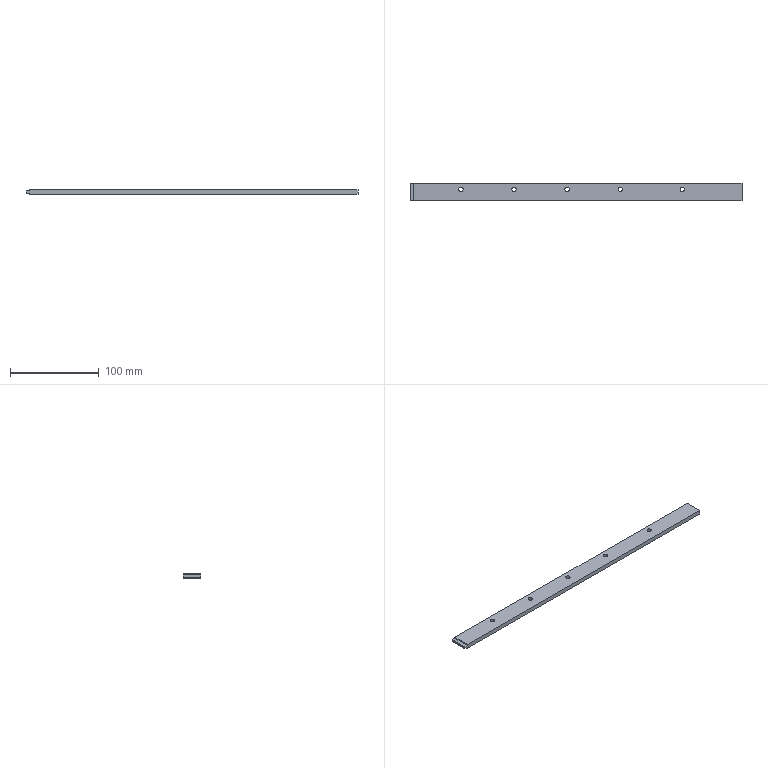Part | STEP file | slingshot press plate | 1 solid | 20 faces | box 375 x 20 x 5 mm | volume 36809 mm3 | cylinder 10 | plane 10 | commonest cylinder face diameters 5 x10
STEP:
#1=CARTESIAN_POINT('',(0.,0.,0.));
#2=DIRECTION('',(0.,0.,1.));
#3=DIRECTION('',(1.,0.,0.));
#4=AXIS2_PLACEMENT_3D('',#1,#2,#3);
#5=CARTESIAN_POINT('',(60.,-7.,0.));
#6=VERTEX_POINT('',#5);
#7=CARTESIAN_POINT('',(60.,-7.,5.));
#8=VERTEX_POINT('',#7);
#9=CARTESIAN_POINT('',(60.,-7.,5.));
#10=DIRECTION('',(0.,0.,1.));
#11=VECTOR('',#10,1.);
#12=LINE('',#9,#11);
#13=CARTESIAN_POINT('',(57.5,-7.,5.));
#14=DIRECTION('',(0.,0.,1.));
#15=DIRECTION('',(1.,0.,0.));
#16=AXIS2_PLACEMENT_3D('',#13,#14,#15);
#17=CYLINDRICAL_SURFACE('',#16,2.5);
#18=CARTESIAN_POINT('',(6.283,0.));
#19=DIRECTION('',(0.,1.));
#20=VECTOR('',#19,1.);
#21=LINE('',#18,#20);
#22=(GEOMETRIC_REPRESENTATION_CONTEXT(2)PARAMETRIC_REPRESENTATION_CONTEXT()REPRESENTATION_CONTEXT('',''));
#23=DEFINITIONAL_REPRESENTATION('',(#21),#22);
#24=PCURVE('',#17,#23);
#25=CARTESIAN_POINT('',(57.5,-7.,5.));
#26=DIRECTION('',(0.,0.,1.));
#27=DIRECTION('',(1.,0.,0.));
#28=AXIS2_PLACEMENT_3D('',#25,#26,#27);
#29=CYLINDRICAL_SURFACE('',#28,2.5);
#30=CARTESIAN_POINT('',(0.,0.));
#31=DIRECTION('',(0.,1.));
#32=VECTOR('',#31,1.);
#33=LINE('',#30,#32);
#34=(GEOMETRIC_REPRESENTATION_CONTEXT(2)PARAMETRIC_REPRESENTATION_CONTEXT()REPRESENTATION_CONTEXT('',''));
#35=DEFINITIONAL_REPRESENTATION('',(#33),#34);
#36=PCURVE('',#29,#35);
#37=SURFACE_CURVE('',#12,(#24,#36),.PCURVE_S1.);
#38=EDGE_CURVE('',#6,#8,#37,.T.);
#39=ORIENTED_EDGE('',*,*,#38,.T.);
#40=CARTESIAN_POINT('',(55.,-7.,5.));
#41=VERTEX_POINT('',#40);
#42=CARTESIAN_POINT('',(57.5,-7.,5.));
#43=DIRECTION('',(0.,0.,1.));
#44=DIRECTION('',(1.,0.,0.));
#45=AXIS2_PLACEMENT_3D('',#42,#43,#44);
#46=CIRCLE('',#45,2.5);
#47=CARTESIAN_POINT('',(0.,0.));
#48=DIRECTION('',(1.,0.));
#49=VECTOR('',#48,1.);
#50=LINE('',#47,#49);
#51=(GEOMETRIC_REPRESENTATION_CONTEXT(2)PARAMETRIC_REPRESENTATION_CONTEXT()REPRESENTATION_CONTEXT('',''));
#52=DEFINITIONAL_REPRESENTATION('',(#50),#51);
#53=PCURVE('',#17,#52);
#54=CARTESIAN_POINT('',(0.,-20.,5.));
#55=DIRECTION('',(0.,0.,1.));
#56=DIRECTION('',(1.,0.,0.));
#57=AXIS2_PLACEMENT_3D('',#54,#55,#56);
#58=PLANE('',#57);
#59=CARTESIAN_POINT('',(57.5,13.));
#60=DIRECTION('',(1.,0.));
#61=AXIS2_PLACEMENT_2D('',#59,#60);
#62=CIRCLE('',#61,2.5);
#63=(GEOMETRIC_REPRESENTATION_CONTEXT(2)PARAMETRIC_REPRESENTATION_CONTEXT()REPRESENTATION_CONTEXT('',''));
#64=DEFINITIONAL_REPRESENTATION('',(#62),#63);
#65=PCURVE('',#58,#64);
#66=SURFACE_CURVE('',#46,(#53,#65),.PCURVE_S1.);
#67=EDGE_CURVE('',#41,#8,#66,.T.);
#68=ORIENTED_EDGE('',*,*,#67,.F.);
#69=CARTESIAN_POINT('',(55.,-7.,0.));
#70=VERTEX_POINT('',#69);
#71=CARTESIAN_POINT('',(55.,-7.,5.));
#72=DIRECTION('',(0.,0.,1.));
#73=VECTOR('',#72,1.);
#74=LINE('',#71,#73);
#75=CARTESIAN_POINT('',(3.142,0.));
#76=DIRECTION('',(0.,1.));
#77=VECTOR('',#76,1.);
#78=LINE('',#75,#77);
#79=(GEOMETRIC_REPRESENTATION_CONTEXT(2)PARAMETRIC_REPRESENTATION_CONTEXT()REPRESENTATION_CONTEXT('',''));
#80=DEFINITIONAL_REPRESENTATION('',(#78),#79);
#81=PCURVE('',#17,#80);
#82=CARTESIAN_POINT('',(3.142,0.));
#83=DIRECTION('',(0.,1.));
#84=VECTOR('',#83,1.);
#85=LINE('',#82,#84);
#86=(GEOMETRIC_REPRESENTATION_CONTEXT(2)PARAMETRIC_REPRESENTATION_CONTEXT()REPRESENTATION_CONTEXT('',''));
#87=DEFINITIONAL_REPRESENTATION('',(#85),#86);
#88=PCURVE('',#29,#87);
#89=SURFACE_CURVE('',#74,(#81,#88),.PCURVE_S1.);
#90=EDGE_CURVE('',#70,#41,#89,.T.);
#91=ORIENTED_EDGE('',*,*,#90,.F.);
#92=CARTESIAN_POINT('',(57.5,-7.,0.));
#93=DIRECTION('',(0.,0.,1.));
#94=DIRECTION('',(1.,0.,0.));
#95=AXIS2_PLACEMENT_3D('',#92,#93,#94);
#96=CIRCLE('',#95,2.5);
#97=CARTESIAN_POINT('',(0.,-5.));
#98=DIRECTION('',(1.,0.));
#99=VECTOR('',#98,1.);
#100=LINE('',#97,#99);
#101=(GEOMETRIC_REPRESENTATION_CONTEXT(2)PARAMETRIC_REPRESENTATION_CONTEXT()REPRESENTATION_CONTEXT('',''));
#102=DEFINITIONAL_REPRESENTATION('',(#100),#101);
#103=PCURVE('',#17,#102);
#104=CARTESIAN_POINT('',(0.,-20.,0.));
#105=DIRECTION('',(0.,0.,1.));
#106=DIRECTION('',(1.,0.,0.));
#107=AXIS2_PLACEMENT_3D('',#104,#105,#106);
#108=PLANE('',#107);
#109=CARTESIAN_POINT('',(57.5,13.));
#110=DIRECTION('',(1.,0.));
#111=AXIS2_PLACEMENT_2D('',#109,#110);
#112=CIRCLE('',#111,2.5);
#113=(GEOMETRIC_REPRESENTATION_CONTEXT(2)PARAMETRIC_REPRESENTATION_CONTEXT()REPRESENTATION_CONTEXT('',''));
#114=DEFINITIONAL_REPRESENTATION('',(#112),#113);
#115=PCURVE('',#108,#114);
#116=SURFACE_CURVE('',#96,(#103,#115),.PCURVE_S1.);
#117=EDGE_CURVE('',#70,#6,#116,.T.);
#118=ORIENTED_EDGE('',*,*,#117,.T.);
#119=EDGE_LOOP('',(#39,#68,#91,#118));
#120=FACE_BOUND('',#119,.F.);
#121=ADVANCED_FACE('',(#120),#17,.F.);
#122=CARTESIAN_POINT('',(120.,-7.,0.));
#123=VERTEX_POINT('',#122);
#124=CARTESIAN_POINT('',(120.,-7.,5.));
#125=VERTEX_POINT('',#124);
#126=CARTESIAN_POINT('',(120.,-7.,5.));
#127=DIRECTION('',(0.,0.,1.));
#128=VECTOR('',#127,1.);
#129=LINE('',#126,#128);
#130=CARTESIAN_POINT('',(117.5,-7.,5.));
#131=DIRECTION('',(0.,0.,1.));
#132=DIRECTION('',(1.,0.,0.));
#133=AXIS2_PLACEMENT_3D('',#130,#131,#132);
#134=CYLINDRICAL_SURFACE('',#133,2.5);
#135=CARTESIAN_POINT('',(6.283,0.));
#136=DIRECTION('',(0.,1.));
#137=VECTOR('',#136,1.);
#138=LINE('',#135,#137);
#139=(GEOMETRIC_REPRESENTATION_CONTEXT(2)PARAMETRIC_REPRESENTATION_CONTEXT()REPRESENTATION_CONTEXT('',''));
#140=DEFINITIONAL_REPRESENTATION('',(#138),#139);
#141=PCURVE('',#134,#140);
#142=CARTESIAN_POINT('',(117.5,-7.,5.));
#143=DIRECTION('',(0.,0.,1.));
#144=DIRECTION('',(1.,0.,0.));
#145=AXIS2_PLACEMENT_3D('',#142,#143,#144);
#146=CYLINDRICAL_SURFACE('',#145,2.5);
#147=CARTESIAN_POINT('',(0.,0.));
#148=DIRECTION('',(0.,1.));
#149=VECTOR('',#148,1.);
#150=LINE('',#147,#149);
#151=(GEOMETRIC_REPRESENTATION_CONTEXT(2)PARAMETRIC_REPRESENTATION_CONTEXT()REPRESENTATION_CONTEXT('',''));
#152=DEFINITIONAL_REPRESENTATION('',(#150),#151);
#153=PCURVE('',#146,#152);
#154=SURFACE_CURVE('',#129,(#141,#153),.PCURVE_S1.);
#155=EDGE_CURVE('',#123,#125,#154,.T.);
#156=ORIENTED_EDGE('',*,*,#155,.T.);
#157=CARTESIAN_POINT('',(115.,-7.,5.));
#158=VERTEX_POINT('',#157);
#159=CARTESIAN_POINT('',(117.5,-7.,5.));
#160=DIRECTION('',(0.,0.,1.));
#161=DIRECTION('',(1.,0.,0.));
#162=AXIS2_PLACEMENT_3D('',#159,#160,#161);
#163=CIRCLE('',#162,2.5);
#164=CARTESIAN_POINT('',(0.,0.));
#165=DIRECTION('',(1.,0.));
#166=VECTOR('',#165,1.);
#167=LINE('',#164,#166);
#168=(GEOMETRIC_REPRESENTATION_CONTEXT(2)PARAMETRIC_REPRESENTATION_CONTEXT()REPRESENTATION_CONTEXT('',''));
#169=DEFINITIONAL_REPRESENTATION('',(#167),#168);
#170=PCURVE('',#134,#169);
#171=CARTESIAN_POINT('',(117.5,13.));
#172=DIRECTION('',(1.,0.));
#173=AXIS2_PLACEMENT_2D('',#171,#172);
#174=CIRCLE('',#173,2.5);
#175=(GEOMETRIC_REPRESENTATION_CONTEXT(2)PARAMETRIC_REPRESENTATION_CONTEXT()REPRESENTATION_CONTEXT('',''));
#176=DEFINITIONAL_REPRESENTATION('',(#174),#175);
#177=PCURVE('',#58,#176);
#178=SURFACE_CURVE('',#163,(#170,#177),.PCURVE_S1.);
#179=EDGE_CURVE('',#158,#125,#178,.T.);
#180=ORIENTED_EDGE('',*,*,#179,.F.);
#181=CARTESIAN_POINT('',(115.,-7.,0.));
#182=VERTEX_POINT('',#181);
#183=CARTESIAN_POINT('',(115.,-7.,5.));
#184=DIRECTION('',(0.,0.,1.));
#185=VECTOR('',#184,1.);
#186=LINE('',#183,#185);
#187=CARTESIAN_POINT('',(3.142,0.));
#188=DIRECTION('',(0.,1.));
#189=VECTOR('',#188,1.);
#190=LINE('',#187,#189);
#191=(GEOMETRIC_REPRESENTATION_CONTEXT(2)PARAMETRIC_REPRESENTATION_CONTEXT()REPRESENTATION_CONTEXT('',''));
#192=DEFINITIONAL_REPRESENTATION('',(#190),#191);
#193=PCURVE('',#134,#192);
#194=CARTESIAN_POINT('',(3.142,0.));
#195=DIRECTION('',(0.,1.));
#196=VECTOR('',#195,1.);
#197=LINE('',#194,#196);
#198=(GEOMETRIC_REPRESENTATION_CONTEXT(2)PARAMETRIC_REPRESENTATION_CONTEXT()REPRESENTATION_CONTEXT('',''));
#199=DEFINITIONAL_REPRESENTATION('',(#197),#198);
#200=PCURVE('',#146,#199);
#201=SURFACE_CURVE('',#186,(#193,#200),.PCURVE_S1.);
#202=EDGE_CURVE('',#182,#158,#201,.T.);
#203=ORIENTED_EDGE('',*,*,#202,.F.);
#204=CARTESIAN_POINT('',(117.5,-7.,0.));
#205=DIRECTION('',(0.,0.,1.));
#206=DIRECTION('',(1.,0.,0.));
#207=AXIS2_PLACEMENT_3D('',#204,#205,#206);
#208=CIRCLE('',#207,2.5);
#209=CARTESIAN_POINT('',(0.,-5.));
#210=DIRECTION('',(1.,0.));
#211=VECTOR('',#210,1.);
#212=LINE('',#209,#211);
#213=(GEOMETRIC_REPRESENTATION_CONTEXT(2)PARAMETRIC_REPRESENTATION_CONTEXT()REPRESENTATION_CONTEXT('',''));
#214=DEFINITIONAL_REPRESENTATION('',(#212),#213);
#215=PCURVE('',#134,#214);
#216=CARTESIAN_POINT('',(117.5,13.));
#217=DIRECTION('',(1.,0.));
#218=AXIS2_PLACEMENT_2D('',#216,#217);
#219=CIRCLE('',#218,2.5);
#220=(GEOMETRIC_REPRESENTATION_CONTEXT(2)PARAMETRIC_REPRESENTATION_CONTEXT()REPRESENTATION_CONTEXT('',''));
#221=DEFINITIONAL_REPRESENTATION('',(#219),#220);
#222=PCURVE('',#108,#221);
#223=SURFACE_CURVE('',#208,(#215,#222),.PCURVE_S1.);
#224=EDGE_CURVE('',#182,#123,#223,.T.);
#225=ORIENTED_EDGE('',*,*,#224,.T.);
#226=EDGE_LOOP('',(#156,#180,#203,#225));
#227=FACE_BOUND('',#226,.F.);
#228=ADVANCED_FACE('',(#227),#134,.F.);
#229=CARTESIAN_POINT('',(180.,-7.,0.));
#230=VERTEX_POINT('',#229);
#231=CARTESIAN_POINT('',(180.,-7.,5.));
#232=VERTEX_POINT('',#231);
#233=CARTESIAN_POINT('',(180.,-7.,5.));
#234=DIRECTION('',(0.,0.,1.));
#235=VECTOR('',#234,1.);
#236=LINE('',#233,#235);
#237=CARTESIAN_POINT('',(177.5,-7.,5.));
#238=DIRECTION('',(0.,0.,1.));
#239=DIRECTION('',(1.,0.,0.));
#240=AXIS2_PLACEMENT_3D('',#237,#238,#239);
#241=CYLINDRICAL_SURFACE('',#240,2.5);
#242=CARTESIAN_POINT('',(6.283,0.));
#243=DIRECTION('',(0.,1.));
#244=VECTOR('',#243,1.);
#245=LINE('',#242,#244);
#246=(GEOMETRIC_REPRESENTATION_CONTEXT(2)PARAMETRIC_REPRESENTATION_CONTEXT()REPRESENTATION_CONTEXT('',''));
#247=DEFINITIONAL_REPRESENTATION('',(#245),#246);
#248=PCURVE('',#241,#247);
#249=CARTESIAN_POINT('',(177.5,-7.,5.));
#250=DIRECTION('',(0.,0.,1.));
#251=DIRECTION('',(1.,0.,0.));
#252=AXIS2_PLACEMENT_3D('',#249,#250,#251);
#253=CYLINDRICAL_SURFACE('',#252,2.5);
#254=CARTESIAN_POINT('',(0.,0.));
#255=DIRECTION('',(0.,1.));
#256=VECTOR('',#255,1.);
#257=LINE('',#254,#256);
#258=(GEOMETRIC_REPRESENTATION_CONTEXT(2)PARAMETRIC_REPRESENTATION_CONTEXT()REPRESENTATION_CONTEXT('',''));
#259=DEFINITIONAL_REPRESENTATION('',(#257),#258);
#260=PCURVE('',#253,#259);
#261=SURFACE_CURVE('',#236,(#248,#260),.PCURVE_S1.);
#262=EDGE_CURVE('',#230,#232,#261,.T.);
#263=ORIENTED_EDGE('',*,*,#262,.T.);
#264=CARTESIAN_POINT('',(175.,-7.,5.));
#265=VERTEX_POINT('',#264);
#266=CARTESIAN_POINT('',(177.5,-7.,5.));
#267=DIRECTION('',(0.,0.,1.));
#268=DIRECTION('',(1.,0.,0.));
#269=AXIS2_PLACEMENT_3D('',#266,#267,#268);
#270=CIRCLE('',#269,2.5);
#271=CARTESIAN_POINT('',(0.,0.));
#272=DIRECTION('',(1.,0.));
#273=VECTOR('',#272,1.);
#274=LINE('',#271,#273);
#275=(GEOMETRIC_REPRESENTATION_CONTEXT(2)PARAMETRIC_REPRESENTATION_CONTEXT()REPRESENTATION_CONTEXT('',''));
#276=DEFINITIONAL_REPRESENTATION('',(#274),#275);
#277=PCURVE('',#241,#276);
#278=CARTESIAN_POINT('',(177.5,13.));
#279=DIRECTION('',(1.,0.));
#280=AXIS2_PLACEMENT_2D('',#278,#279);
#281=CIRCLE('',#280,2.5);
#282=(GEOMETRIC_REPRESENTATION_CONTEXT(2)PARAMETRIC_REPRESENTATION_CONTEXT()REPRESENTATION_CONTEXT('',''));
#283=DEFINITIONAL_REPRESENTATION('',(#281),#282);
#284=PCURVE('',#58,#283);
#285=SURFACE_CURVE('',#270,(#277,#284),.PCURVE_S1.);
#286=EDGE_CURVE('',#265,#232,#285,.T.);
#287=ORIENTED_EDGE('',*,*,#286,.F.);
#288=CARTESIAN_POINT('',(175.,-7.,0.));
#289=VERTEX_POINT('',#288);
#290=CARTESIAN_POINT('',(175.,-7.,5.));
#291=DIRECTION('',(0.,0.,1.));
#292=VECTOR('',#291,1.);
#293=LINE('',#290,#292);
#294=CARTESIAN_POINT('',(3.142,0.));
#295=DIRECTION('',(0.,1.));
#296=VECTOR('',#295,1.);
#297=LINE('',#294,#296);
#298=(GEOMETRIC_REPRESENTATION_CONTEXT(2)PARAMETRIC_REPRESENTATION_CONTEXT()REPRESENTATION_CONTEXT('',''));
#299=DEFINITIONAL_REPRESENTATION('',(#297),#298);
#300=PCURVE('',#241,#299);
#301=CARTESIAN_POINT('',(3.142,0.));
#302=DIRECTION('',(0.,1.));
#303=VECTOR('',#302,1.);
#304=LINE('',#301,#303);
#305=(GEOMETRIC_REPRESENTATION_CONTEXT(2)PARAMETRIC_REPRESENTATION_CONTEXT()REPRESENTATION_CONTEXT('',''));
#306=DEFINITIONAL_REPRESENTATION('',(#304),#305);
#307=PCURVE('',#253,#306);
#308=SURFACE_CURVE('',#293,(#300,#307),.PCURVE_S1.);
#309=EDGE_CURVE('',#289,#265,#308,.T.);
#310=ORIENTED_EDGE('',*,*,#309,.F.);
#311=CARTESIAN_POINT('',(177.5,-7.,0.));
#312=DIRECTION('',(0.,0.,1.));
#313=DIRECTION('',(1.,0.,0.));
#314=AXIS2_PLACEMENT_3D('',#311,#312,#313);
#315=CIRCLE('',#314,2.5);
#316=CARTESIAN_POINT('',(0.,-5.));
#317=DIRECTION('',(1.,0.));
#318=VECTOR('',#317,1.);
#319=LINE('',#316,#318);
#320=(GEOMETRIC_REPRESENTATION_CONTEXT(2)PARAMETRIC_REPRESENTATION_CONTEXT()REPRESENTATION_CONTEXT('',''));
#321=DEFINITIONAL_REPRESENTATION('',(#319),#320);
#322=PCURVE('',#241,#321);
#323=CARTESIAN_POINT('',(177.5,13.));
#324=DIRECTION('',(1.,0.));
#325=AXIS2_PLACEMENT_2D('',#323,#324);
#326=CIRCLE('',#325,2.5);
#327=(GEOMETRIC_REPRESENTATION_CONTEXT(2)PARAMETRIC_REPRESENTATION_CONTEXT()REPRESENTATION_CONTEXT('',''));
#328=DEFINITIONAL_REPRESENTATION('',(#326),#327);
#329=PCURVE('',#108,#328);
#330=SURFACE_CURVE('',#315,(#322,#329),.PCURVE_S1.);
#331=EDGE_CURVE('',#289,#230,#330,.T.);
#332=ORIENTED_EDGE('',*,*,#331,.T.);
#333=EDGE_LOOP('',(#263,#287,#310,#332));
#334=FACE_BOUND('',#333,.F.);
#335=ADVANCED_FACE('',(#334),#241,.F.);
#336=CARTESIAN_POINT('',(240.,-7.,0.));
#337=VERTEX_POINT('',#336);
#338=CARTESIAN_POINT('',(240.,-7.,5.));
#339=VERTEX_POINT('',#338);
#340=CARTESIAN_POINT('',(240.,-7.,5.));
#341=DIRECTION('',(0.,0.,1.));
#342=VECTOR('',#341,1.);
#343=LINE('',#340,#342);
#344=CARTESIAN_POINT('',(237.5,-7.,5.));
#345=DIRECTION('',(0.,0.,1.));
#346=DIRECTION('',(1.,0.,0.));
#347=AXIS2_PLACEMENT_3D('',#344,#345,#346);
#348=CYLINDRICAL_SURFACE('',#347,2.5);
#349=CARTESIAN_POINT('',(6.283,0.));
#350=DIRECTION('',(0.,1.));
#351=VECTOR('',#350,1.);
#352=LINE('',#349,#351);
#353=(GEOMETRIC_REPRESENTATION_CONTEXT(2)PARAMETRIC_REPRESENTATION_CONTEXT()REPRESENTATION_CONTEXT('',''));
#354=DEFINITIONAL_REPRESENTATION('',(#352),#353);
#355=PCURVE('',#348,#354);
#356=CARTESIAN_POINT('',(237.5,-7.,5.));
#357=DIRECTION('',(0.,0.,1.));
#358=DIRECTION('',(1.,0.,0.));
#359=AXIS2_PLACEMENT_3D('',#356,#357,#358);
#360=CYLINDRICAL_SURFACE('',#359,2.5);
#361=CARTESIAN_POINT('',(0.,0.));
#362=DIRECTION('',(0.,1.));
#363=VECTOR('',#362,1.);
#364=LINE('',#361,#363);
#365=(GEOMETRIC_REPRESENTATION_CONTEXT(2)PARAMETRIC_REPRESENTATION_CONTEXT()REPRESENTATION_CONTEXT('',''));
#366=DEFINITIONAL_REPRESENTATION('',(#364),#365);
#367=PCURVE('',#360,#366);
#368=SURFACE_CURVE('',#343,(#355,#367),.PCURVE_S1.);
#369=EDGE_CURVE('',#337,#339,#368,.T.);
#370=ORIENTED_EDGE('',*,*,#369,.T.);
#371=CARTESIAN_POINT('',(235.,-7.,5.));
#372=VERTEX_POINT('',#371);
#373=CARTESIAN_POINT('',(237.5,-7.,5.));
#374=DIRECTION('',(0.,0.,1.));
#375=DIRECTION('',(1.,0.,0.));
#376=AXIS2_PLACEMENT_3D('',#373,#374,#375);
#377=CIRCLE('',#376,2.5);
#378=CARTESIAN_POINT('',(0.,0.));
#379=DIRECTION('',(1.,0.));
#380=VECTOR('',#379,1.);
#381=LINE('',#378,#380);
#382=(GEOMETRIC_REPRESENTATION_CONTEXT(2)PARAMETRIC_REPRESENTATION_CONTEXT()REPRESENTATION_CONTEXT('',''));
#383=DEFINITIONAL_REPRESENTATION('',(#381),#382);
#384=PCURVE('',#348,#383);
#385=CARTESIAN_POINT('',(237.5,13.));
#386=DIRECTION('',(1.,0.));
#387=AXIS2_PLACEMENT_2D('',#385,#386);
#388=CIRCLE('',#387,2.5);
#389=(GEOMETRIC_REPRESENTATION_CONTEXT(2)PARAMETRIC_REPRESENTATION_CONTEXT()REPRESENTATION_CONTEXT('',''));
#390=DEFINITIONAL_REPRESENTATION('',(#388),#389);
#391=PCURVE('',#58,#390);
#392=SURFACE_CURVE('',#377,(#384,#391),.PCURVE_S1.);
#393=EDGE_CURVE('',#372,#339,#392,.T.);
#394=ORIENTED_EDGE('',*,*,#393,.F.);
#395=CARTESIAN_POINT('',(235.,-7.,0.));
#396=VERTEX_POINT('',#395);
#397=CARTESIAN_POINT('',(235.,-7.,5.));
#398=DIRECTION('',(0.,0.,1.));
#399=VECTOR('',#398,1.);
#400=LINE('',#397,#399);
#401=CARTESIAN_POINT('',(3.142,0.));
#402=DIRECTION('',(0.,1.));
#403=VECTOR('',#402,1.);
#404=LINE('',#401,#403);
#405=(GEOMETRIC_REPRESENTATION_CONTEXT(2)PARAMETRIC_REPRESENTATION_CONTEXT()REPRESENTATION_CONTEXT('',''));
#406=DEFINITIONAL_REPRESENTATION('',(#404),#405);
#407=PCURVE('',#348,#406);
#408=CARTESIAN_POINT('',(3.142,0.));
#409=DIRECTION('',(0.,1.));
#410=VECTOR('',#409,1.);
#411=LINE('',#408,#410);
#412=(GEOMETRIC_REPRESENTATION_CONTEXT(2)PARAMETRIC_REPRESENTATION_CONTEXT()REPRESENTATION_CONTEXT('',''));
#413=DEFINITIONAL_REPRESENTATION('',(#411),#412);
#414=PCURVE('',#360,#413);
#415=SURFACE_CURVE('',#400,(#407,#414),.PCURVE_S1.);
#416=EDGE_CURVE('',#396,#372,#415,.T.);
#417=ORIENTED_EDGE('',*,*,#416,.F.);
#418=CARTESIAN_POINT('',(237.5,-7.,0.));
#419=DIRECTION('',(0.,0.,1.));
#420=DIRECTION('',(1.,0.,0.));
#421=AXIS2_PLACEMENT_3D('',#418,#419,#420);
#422=CIRCLE('',#421,2.5);
#423=CARTESIAN_POINT('',(0.,-5.));
#424=DIRECTION('',(1.,0.));
#425=VECTOR('',#424,1.);
#426=LINE('',#423,#425);
#427=(GEOMETRIC_REPRESENTATION_CONTEXT(2)PARAMETRIC_REPRESENTATION_CONTEXT()REPRESENTATION_CONTEXT('',''));
#428=DEFINITIONAL_REPRESENTATION('',(#426),#427);
#429=PCURVE('',#348,#428);
#430=CARTESIAN_POINT('',(237.5,13.));
#431=DIRECTION('',(1.,0.));
#432=AXIS2_PLACEMENT_2D('',#430,#431);
#433=CIRCLE('',#432,2.5);
#434=(GEOMETRIC_REPRESENTATION_CONTEXT(2)PARAMETRIC_REPRESENTATION_CONTEXT()REPRESENTATION_CONTEXT('',''));
#435=DEFINITIONAL_REPRESENTATION('',(#433),#434);
#436=PCURVE('',#108,#435);
#437=SURFACE_CURVE('',#422,(#429,#436),.PCURVE_S1.);
#438=EDGE_CURVE('',#396,#337,#437,.T.);
#439=ORIENTED_EDGE('',*,*,#438,.T.);
#440=EDGE_LOOP('',(#370,#394,#417,#439));
#441=FACE_BOUND('',#440,.F.);
#442=ADVANCED_FACE('',(#441),#348,.F.);
#443=CARTESIAN_POINT('',(310.,-7.,0.));
#444=VERTEX_POINT('',#443);
#445=CARTESIAN_POINT('',(310.,-7.,5.));
#446=VERTEX_POINT('',#445);
#447=CARTESIAN_POINT('',(310.,-7.,5.));
#448=DIRECTION('',(0.,0.,1.));
#449=VECTOR('',#448,1.);
#450=LINE('',#447,#449);
#451=CARTESIAN_POINT('',(307.5,-7.,5.));
#452=DIRECTION('',(0.,0.,1.));
#453=DIRECTION('',(1.,0.,0.));
#454=AXIS2_PLACEMENT_3D('',#451,#452,#453);
#455=CYLINDRICAL_SURFACE('',#454,2.5);
#456=CARTESIAN_POINT('',(6.283,0.));
#457=DIRECTION('',(0.,1.));
#458=VECTOR('',#457,1.);
#459=LINE('',#456,#458);
#460=(GEOMETRIC_REPRESENTATION_CONTEXT(2)PARAMETRIC_REPRESENTATION_CONTEXT()REPRESENTATION_CONTEXT('',''));
#461=DEFINITIONAL_REPRESENTATION('',(#459),#460);
#462=PCURVE('',#455,#461);
#463=CARTESIAN_POINT('',(307.5,-7.,5.));
#464=DIRECTION('',(0.,0.,1.));
#465=DIRECTION('',(1.,0.,0.));
#466=AXIS2_PLACEMENT_3D('',#463,#464,#465);
#467=CYLINDRICAL_SURFACE('',#466,2.5);
#468=CARTESIAN_POINT('',(0.,0.));
#469=DIRECTION('',(0.,1.));
#470=VECTOR('',#469,1.);
#471=LINE('',#468,#470);
#472=(GEOMETRIC_REPRESENTATION_CONTEXT(2)PARAMETRIC_REPRESENTATION_CONTEXT()REPRESENTATION_CONTEXT('',''));
#473=DEFINITIONAL_REPRESENTATION('',(#471),#472);
#474=PCURVE('',#467,#473);
#475=SURFACE_CURVE('',#450,(#462,#474),.PCURVE_S1.);
#476=EDGE_CURVE('',#444,#446,#475,.T.);
#477=ORIENTED_EDGE('',*,*,#476,.T.);
#478=CARTESIAN_POINT('',(305.,-7.,5.));
#479=VERTEX_POINT('',#478);
#480=CARTESIAN_POINT('',(307.5,-7.,5.));
#481=DIRECTION('',(0.,0.,1.));
#482=DIRECTION('',(1.,0.,0.));
#483=AXIS2_PLACEMENT_3D('',#480,#481,#482);
#484=CIRCLE('',#483,2.5);
#485=CARTESIAN_POINT('',(0.,0.));
#486=DIRECTION('',(1.,0.));
#487=VECTOR('',#486,1.);
#488=LINE('',#485,#487);
#489=(GEOMETRIC_REPRESENTATION_CONTEXT(2)PARAMETRIC_REPRESENTATION_CONTEXT()REPRESENTATION_CONTEXT('',''));
#490=DEFINITIONAL_REPRESENTATION('',(#488),#489);
#491=PCURVE('',#455,#490);
#492=CARTESIAN_POINT('',(307.5,13.));
#493=DIRECTION('',(1.,0.));
#494=AXIS2_PLACEMENT_2D('',#492,#493);
#495=CIRCLE('',#494,2.5);
#496=(GEOMETRIC_REPRESENTATION_CONTEXT(2)PARAMETRIC_REPRESENTATION_CONTEXT()REPRESENTATION_CONTEXT('',''));
#497=DEFINITIONAL_REPRESENTATION('',(#495),#496);
#498=PCURVE('',#58,#497);
#499=SURFACE_CURVE('',#484,(#491,#498),.PCURVE_S1.);
#500=EDGE_CURVE('',#479,#446,#499,.T.);
#501=ORIENTED_EDGE('',*,*,#500,.F.);
#502=CARTESIAN_POINT('',(305.,-7.,0.));
#503=VERTEX_POINT('',#502);
#504=CARTESIAN_POINT('',(305.,-7.,5.));
#505=DIRECTION('',(0.,0.,1.));
#506=VECTOR('',#505,1.);
#507=LINE('',#504,#506);
#508=CARTESIAN_POINT('',(3.142,0.));
#509=DIRECTION('',(0.,1.));
#510=VECTOR('',#509,1.);
#511=LINE('',#508,#510);
#512=(GEOMETRIC_REPRESENTATION_CONTEXT(2)PARAMETRIC_REPRESENTATION_CONTEXT()REPRESENTATION_CONTEXT('',''));
#513=DEFINITIONAL_REPRESENTATION('',(#511),#512);
#514=PCURVE('',#455,#513);
#515=CARTESIAN_POINT('',(3.142,0.));
#516=DIRECTION('',(0.,1.));
#517=VECTOR('',#516,1.);
#518=LINE('',#515,#517);
#519=(GEOMETRIC_REPRESENTATION_CONTEXT(2)PARAMETRIC_REPRESENTATION_CONTEXT()REPRESENTATION_CONTEXT('',''));
#520=DEFINITIONAL_REPRESENTATION('',(#518),#519);
#521=PCURVE('',#467,#520);
#522=SURFACE_CURVE('',#507,(#514,#521),.PCURVE_S1.);
#523=EDGE_CURVE('',#503,#479,#522,.T.);
#524=ORIENTED_EDGE('',*,*,#523,.F.);
#525=CARTESIAN_POINT('',(307.5,-7.,0.));
#526=DIRECTION('',(0.,0.,1.));
#527=DIRECTION('',(1.,0.,0.));
#528=AXIS2_PLACEMENT_3D('',#525,#526,#527);
#529=CIRCLE('',#528,2.5);
#530=CARTESIAN_POINT('',(0.,-5.));
#531=DIRECTION('',(1.,0.));
#532=VECTOR('',#531,1.);
#533=LINE('',#530,#532);
#534=(GEOMETRIC_REPRESENTATION_CONTEXT(2)PARAMETRIC_REPRESENTATION_CONTEXT()REPRESENTATION_CONTEXT('',''));
#535=DEFINITIONAL_REPRESENTATION('',(#533),#534);
#536=PCURVE('',#455,#535);
#537=CARTESIAN_POINT('',(307.5,13.));
#538=DIRECTION('',(1.,0.));
#539=AXIS2_PLACEMENT_2D('',#537,#538);
#540=CIRCLE('',#539,2.5);
#541=(GEOMETRIC_REPRESENTATION_CONTEXT(2)PARAMETRIC_REPRESENTATION_CONTEXT()REPRESENTATION_CONTEXT('',''));
#542=DEFINITIONAL_REPRESENTATION('',(#540),#541);
#543=PCURVE('',#108,#542);
#544=SURFACE_CURVE('',#529,(#536,#543),.PCURVE_S1.);
#545=EDGE_CURVE('',#503,#444,#544,.T.);
#546=ORIENTED_EDGE('',*,*,#545,.T.);
#547=EDGE_LOOP('',(#477,#501,#524,#546));
#548=FACE_BOUND('',#547,.F.);
#549=ADVANCED_FACE('',(#548),#455,.F.);
#550=CARTESIAN_POINT('',(0.,-20.,1.25));
#551=VERTEX_POINT('',#550);
#552=CARTESIAN_POINT('',(0.,0.,1.25));
#553=VERTEX_POINT('',#552);
#554=CARTESIAN_POINT('',(0.,0.,1.25));
#555=DIRECTION('',(0.,1.,0.));
#556=VECTOR('',#555,1.);
#557=LINE('',#554,#556);
#558=CARTESIAN_POINT('',(0.,0.,5.));
#559=DIRECTION('',(1.,0.,0.));
#560=DIRECTION('',(0.,1.,0.));
#561=AXIS2_PLACEMENT_3D('',#558,#559,#560);
#562=PLANE('',#561);
#563=CARTESIAN_POINT('',(0.,-3.75));
#564=DIRECTION('',(1.,0.));
#565=VECTOR('',#564,1.);
#566=LINE('',#563,#565);
#567=(GEOMETRIC_REPRESENTATION_CONTEXT(2)PARAMETRIC_REPRESENTATION_CONTEXT()REPRESENTATION_CONTEXT('',''));
#568=DEFINITIONAL_REPRESENTATION('',(#566),#567);
#569=PCURVE('',#562,#568);
#570=CARTESIAN_POINT('',(4.,-32.927,1.25));
#571=DIRECTION('',(0.,0.,-1.));
#572=DIRECTION('',(-1.,0.,0.));
#573=AXIS2_PLACEMENT_3D('',#570,#571,#572);
#574=PLANE('',#573);
#575=CARTESIAN_POINT('',(4.,32.927));
#576=DIRECTION('',(0.,1.));
#577=VECTOR('',#576,1.);
#578=LINE('',#575,#577);
#579=(GEOMETRIC_REPRESENTATION_CONTEXT(2)PARAMETRIC_REPRESENTATION_CONTEXT()REPRESENTATION_CONTEXT('',''));
#580=DEFINITIONAL_REPRESENTATION('',(#578),#579);
#581=PCURVE('',#574,#580);
#582=SURFACE_CURVE('',#557,(#569,#581),.PCURVE_S1.);
#583=EDGE_CURVE('',#551,#553,#582,.T.);
#584=ORIENTED_EDGE('',*,*,#583,.F.);
#585=CARTESIAN_POINT('',(0.,-20.,3.75));
#586=VERTEX_POINT('',#585);
#587=CARTESIAN_POINT('',(0.,-20.,5.));
#588=DIRECTION('',(0.,0.,-1.));
#589=VECTOR('',#588,1.);
#590=LINE('',#587,#589);
#591=CARTESIAN_POINT('',(-20.,0.));
#592=DIRECTION('',(0.,-1.));
#593=VECTOR('',#592,1.);
#594=LINE('',#591,#593);
#595=(GEOMETRIC_REPRESENTATION_CONTEXT(2)PARAMETRIC_REPRESENTATION_CONTEXT()REPRESENTATION_CONTEXT('',''));
#596=DEFINITIONAL_REPRESENTATION('',(#594),#595);
#597=PCURVE('',#562,#596);
#598=CARTESIAN_POINT('',(0.,-20.,5.));
#599=DIRECTION('',(0.,1.,0.));
#600=DIRECTION('',(0.,0.,1.));
#601=AXIS2_PLACEMENT_3D('',#598,#599,#600);
#602=PLANE('',#601);
#603=CARTESIAN_POINT('',(0.,0.));
#604=DIRECTION('',(-1.,0.));
#605=VECTOR('',#604,1.);
#606=LINE('',#603,#605);
#607=(GEOMETRIC_REPRESENTATION_CONTEXT(2)PARAMETRIC_REPRESENTATION_CONTEXT()REPRESENTATION_CONTEXT('',''));
#608=DEFINITIONAL_REPRESENTATION('',(#606),#607);
#609=PCURVE('',#602,#608);
#610=SURFACE_CURVE('',#590,(#597,#609),.PCURVE_S1.);
#611=EDGE_CURVE('',#586,#551,#610,.T.);
#612=ORIENTED_EDGE('',*,*,#611,.F.);
#613=CARTESIAN_POINT('',(0.,0.,3.75));
#614=VERTEX_POINT('',#613);
#615=CARTESIAN_POINT('',(0.,0.,3.75));
#616=DIRECTION('',(0.,1.,0.));
#617=VECTOR('',#616,1.);
#618=LINE('',#615,#617);
#619=CARTESIAN_POINT('',(0.,-1.25));
#620=DIRECTION('',(1.,0.));
#621=VECTOR('',#620,1.);
#622=LINE('',#619,#621);
#623=(GEOMETRIC_REPRESENTATION_CONTEXT(2)PARAMETRIC_REPRESENTATION_CONTEXT()REPRESENTATION_CONTEXT('',''));
#624=DEFINITIONAL_REPRESENTATION('',(#622),#623);
#625=PCURVE('',#562,#624);
#626=CARTESIAN_POINT('',(-14.006,5.289,3.75));
#627=DIRECTION('',(0.,0.,-1.));
#628=DIRECTION('',(-1.,0.,0.));
#629=AXIS2_PLACEMENT_3D('',#626,#627,#628);
#630=PLANE('',#629);
#631=CARTESIAN_POINT('',(-14.006,-5.289));
#632=DIRECTION('',(0.,1.));
#633=VECTOR('',#632,1.);
#634=LINE('',#631,#633);
#635=(GEOMETRIC_REPRESENTATION_CONTEXT(2)PARAMETRIC_REPRESENTATION_CONTEXT()REPRESENTATION_CONTEXT('',''));
#636=DEFINITIONAL_REPRESENTATION('',(#634),#635);
#637=PCURVE('',#630,#636);
#638=SURFACE_CURVE('',#618,(#625,#637),.PCURVE_S1.);
#639=EDGE_CURVE('',#586,#614,#638,.T.);
#640=ORIENTED_EDGE('',*,*,#639,.T.);
#641=CARTESIAN_POINT('',(0.,0.,5.));
#642=DIRECTION('',(0.,0.,-1.));
#643=VECTOR('',#642,1.);
#644=LINE('',#641,#643);
#645=CARTESIAN_POINT('',(0.,0.));
#646=DIRECTION('',(0.,-1.));
#647=VECTOR('',#646,1.);
#648=LINE('',#645,#647);
#649=(GEOMETRIC_REPRESENTATION_CONTEXT(2)PARAMETRIC_REPRESENTATION_CONTEXT()REPRESENTATION_CONTEXT('',''));
#650=DEFINITIONAL_REPRESENTATION('',(#648),#649);
#651=PCURVE('',#562,#650);
#652=CARTESIAN_POINT('',(0.,0.,5.));
#653=DIRECTION('',(0.,-1.,0.));
#654=DIRECTION('',(0.,0.,-1.));
#655=AXIS2_PLACEMENT_3D('',#652,#653,#654);
#656=PLANE('',#655);
#657=CARTESIAN_POINT('',(0.,0.));
#658=DIRECTION('',(1.,0.));
#659=VECTOR('',#658,1.);
#660=LINE('',#657,#659);
#661=(GEOMETRIC_REPRESENTATION_CONTEXT(2)PARAMETRIC_REPRESENTATION_CONTEXT()REPRESENTATION_CONTEXT('',''));
#662=DEFINITIONAL_REPRESENTATION('',(#660),#661);
#663=PCURVE('',#656,#662);
#664=SURFACE_CURVE('',#644,(#651,#663),.PCURVE_S1.);
#665=EDGE_CURVE('',#614,#553,#664,.T.);
#666=ORIENTED_EDGE('',*,*,#665,.T.);
#667=EDGE_LOOP('',(#584,#612,#640,#666));
#668=FACE_BOUND('',#667,.T.);
#669=ADVANCED_FACE('',(#668),#562,.F.);
#670=CARTESIAN_POINT('',(4.,-20.,1.25));
#671=VERTEX_POINT('',#670);
#672=CARTESIAN_POINT('',(0.,-20.,1.25));
#673=DIRECTION('',(-1.,0.,0.));
#674=VECTOR('',#673,1.);
#675=LINE('',#672,#674);
#676=CARTESIAN_POINT('',(-3.75,0.));
#677=DIRECTION('',(0.,-1.));
#678=VECTOR('',#677,1.);
#679=LINE('',#676,#678);
#680=(GEOMETRIC_REPRESENTATION_CONTEXT(2)PARAMETRIC_REPRESENTATION_CONTEXT()REPRESENTATION_CONTEXT('',''));
#681=DEFINITIONAL_REPRESENTATION('',(#679),#680);
#682=PCURVE('',#602,#681);
#683=CARTESIAN_POINT('',(4.,12.927));
#684=DIRECTION('',(1.,0.));
#685=VECTOR('',#684,1.);
#686=LINE('',#683,#685);
#687=(GEOMETRIC_REPRESENTATION_CONTEXT(2)PARAMETRIC_REPRESENTATION_CONTEXT()REPRESENTATION_CONTEXT('',''));
#688=DEFINITIONAL_REPRESENTATION('',(#686),#687);
#689=PCURVE('',#574,#688);
#690=SURFACE_CURVE('',#675,(#682,#689),.PCURVE_S1.);
#691=EDGE_CURVE('',#671,#551,#690,.T.);
#692=ORIENTED_EDGE('',*,*,#691,.F.);
#693=CARTESIAN_POINT('',(4.,-20.,0.));
#694=VERTEX_POINT('',#693);
#695=CARTESIAN_POINT('',(4.,-20.,5.));
#696=DIRECTION('',(0.,0.,-1.));
#697=VECTOR('',#696,1.);
#698=LINE('',#695,#697);
#699=CARTESIAN_POINT('',(0.,4.));
#700=DIRECTION('',(-1.,0.));
#701=VECTOR('',#700,1.);
#702=LINE('',#699,#701);
#703=(GEOMETRIC_REPRESENTATION_CONTEXT(2)PARAMETRIC_REPRESENTATION_CONTEXT()REPRESENTATION_CONTEXT('',''));
#704=DEFINITIONAL_REPRESENTATION('',(#702),#703);
#705=PCURVE('',#602,#704);
#706=CARTESIAN_POINT('',(4.,9.518,1.25));
#707=DIRECTION('',(1.,0.,0.));
#708=DIRECTION('',(0.,1.,0.));
#709=AXIS2_PLACEMENT_3D('',#706,#707,#708);
#710=PLANE('',#709);
#711=CARTESIAN_POINT('',(-29.518,3.75));
#712=DIRECTION('',(0.,-1.));
#713=VECTOR('',#712,1.);
#714=LINE('',#711,#713);
#715=(GEOMETRIC_REPRESENTATION_CONTEXT(2)PARAMETRIC_REPRESENTATION_CONTEXT()REPRESENTATION_CONTEXT('',''));
#716=DEFINITIONAL_REPRESENTATION('',(#714),#715);
#717=PCURVE('',#710,#716);
#718=SURFACE_CURVE('',#698,(#705,#717),.PCURVE_S1.);
#719=EDGE_CURVE('',#671,#694,#718,.T.);
#720=ORIENTED_EDGE('',*,*,#719,.T.);
#721=CARTESIAN_POINT('',(375.,-20.,0.));
#722=VERTEX_POINT('',#721);
#723=CARTESIAN_POINT('',(0.,-20.,0.));
#724=DIRECTION('',(1.,0.,0.));
#725=VECTOR('',#724,1.);
#726=LINE('',#723,#725);
#727=CARTESIAN_POINT('',(-5.,0.));
#728=DIRECTION('',(0.,1.));
#729=VECTOR('',#728,1.);
#730=LINE('',#727,#729);
#731=(GEOMETRIC_REPRESENTATION_CONTEXT(2)PARAMETRIC_REPRESENTATION_CONTEXT()REPRESENTATION_CONTEXT('',''));
#732=DEFINITIONAL_REPRESENTATION('',(#730),#731);
#733=PCURVE('',#602,#732);
#734=CARTESIAN_POINT('',(0.,0.));
#735=DIRECTION('',(1.,0.));
#736=VECTOR('',#735,1.);
#737=LINE('',#734,#736);
#738=(GEOMETRIC_REPRESENTATION_CONTEXT(2)PARAMETRIC_REPRESENTATION_CONTEXT()REPRESENTATION_CONTEXT('',''));
#739=DEFINITIONAL_REPRESENTATION('',(#737),#738);
#740=PCURVE('',#108,#739);
#741=SURFACE_CURVE('',#726,(#733,#740),.PCURVE_S1.);
#742=EDGE_CURVE('',#694,#722,#741,.T.);
#743=ORIENTED_EDGE('',*,*,#742,.T.);
#744=CARTESIAN_POINT('',(375.,-20.,5.));
#745=VERTEX_POINT('',#744);
#746=CARTESIAN_POINT('',(375.,-20.,5.));
#747=DIRECTION('',(0.,0.,-1.));
#748=VECTOR('',#747,1.);
#749=LINE('',#746,#748);
#750=CARTESIAN_POINT('',(0.,375.));
#751=DIRECTION('',(-1.,0.));
#752=VECTOR('',#751,1.);
#753=LINE('',#750,#752);
#754=(GEOMETRIC_REPRESENTATION_CONTEXT(2)PARAMETRIC_REPRESENTATION_CONTEXT()REPRESENTATION_CONTEXT('',''));
#755=DEFINITIONAL_REPRESENTATION('',(#753),#754);
#756=PCURVE('',#602,#755);
#757=CARTESIAN_POINT('',(375.,0.,5.));
#758=DIRECTION('',(-1.,0.,0.));
#759=DIRECTION('',(0.,0.,1.));
#760=AXIS2_PLACEMENT_3D('',#757,#758,#759);
#761=PLANE('',#760);
#762=CARTESIAN_POINT('',(0.,-20.));
#763=DIRECTION('',(-1.,0.));
#764=VECTOR('',#763,1.);
#765=LINE('',#762,#764);
#766=(GEOMETRIC_REPRESENTATION_CONTEXT(2)PARAMETRIC_REPRESENTATION_CONTEXT()REPRESENTATION_CONTEXT('',''));
#767=DEFINITIONAL_REPRESENTATION('',(#765),#766);
#768=PCURVE('',#761,#767);
#769=SURFACE_CURVE('',#749,(#756,#768),.PCURVE_S1.);
#770=EDGE_CURVE('',#745,#722,#769,.T.);
#771=ORIENTED_EDGE('',*,*,#770,.F.);
#772=CARTESIAN_POINT('',(4.,-20.,5.));
#773=VERTEX_POINT('',#772);
#774=CARTESIAN_POINT('',(0.,-20.,5.));
#775=DIRECTION('',(1.,0.,0.));
#776=VECTOR('',#775,1.);
#777=LINE('',#774,#776);
#778=CARTESIAN_POINT('',(0.,0.));
#779=DIRECTION('',(0.,1.));
#780=VECTOR('',#779,1.);
#781=LINE('',#778,#780);
#782=(GEOMETRIC_REPRESENTATION_CONTEXT(2)PARAMETRIC_REPRESENTATION_CONTEXT()REPRESENTATION_CONTEXT('',''));
#783=DEFINITIONAL_REPRESENTATION('',(#781),#782);
#784=PCURVE('',#602,#783);
#785=CARTESIAN_POINT('',(0.,0.));
#786=DIRECTION('',(1.,0.));
#787=VECTOR('',#786,1.);
#788=LINE('',#785,#787);
#789=(GEOMETRIC_REPRESENTATION_CONTEXT(2)PARAMETRIC_REPRESENTATION_CONTEXT()REPRESENTATION_CONTEXT('',''));
#790=DEFINITIONAL_REPRESENTATION('',(#788),#789);
#791=PCURVE('',#58,#790);
#792=SURFACE_CURVE('',#777,(#784,#791),.PCURVE_S1.);
#793=EDGE_CURVE('',#773,#745,#792,.T.);
#794=ORIENTED_EDGE('',*,*,#793,.F.);
#795=CARTESIAN_POINT('',(4.,-20.,3.75));
#796=VERTEX_POINT('',#795);
#797=CARTESIAN_POINT('',(4.,-20.,5.));
#798=DIRECTION('',(0.,0.,-1.));
#799=VECTOR('',#798,1.);
#800=LINE('',#797,#799);
#801=CARTESIAN_POINT('',(0.,4.));
#802=DIRECTION('',(-1.,0.));
#803=VECTOR('',#802,1.);
#804=LINE('',#801,#803);
#805=(GEOMETRIC_REPRESENTATION_CONTEXT(2)PARAMETRIC_REPRESENTATION_CONTEXT()REPRESENTATION_CONTEXT('',''));
#806=DEFINITIONAL_REPRESENTATION('',(#804),#805);
#807=PCURVE('',#602,#806);
#808=CARTESIAN_POINT('',(4.,-25.592,3.75));
#809=DIRECTION('',(1.,0.,0.));
#810=DIRECTION('',(0.,0.,-1.));
#811=AXIS2_PLACEMENT_3D('',#808,#809,#810);
#812=PLANE('',#811);
#813=CARTESIAN_POINT('',(-1.25,5.592));
#814=DIRECTION('',(1.,0.));
#815=VECTOR('',#814,1.);
#816=LINE('',#813,#815);
#817=(GEOMETRIC_REPRESENTATION_CONTEXT(2)PARAMETRIC_REPRESENTATION_CONTEXT()REPRESENTATION_CONTEXT('',''));
#818=DEFINITIONAL_REPRESENTATION('',(#816),#817);
#819=PCURVE('',#812,#818);
#820=SURFACE_CURVE('',#800,(#807,#819),.PCURVE_S1.);
#821=EDGE_CURVE('',#773,#796,#820,.T.);
#822=ORIENTED_EDGE('',*,*,#821,.T.);
#823=CARTESIAN_POINT('',(0.,-20.,3.75));
#824=DIRECTION('',(-1.,0.,0.));
#825=VECTOR('',#824,1.);
#826=LINE('',#823,#825);
#827=CARTESIAN_POINT('',(-1.25,0.));
#828=DIRECTION('',(0.,-1.));
#829=VECTOR('',#828,1.);
#830=LINE('',#827,#829);
#831=(GEOMETRIC_REPRESENTATION_CONTEXT(2)PARAMETRIC_REPRESENTATION_CONTEXT()REPRESENTATION_CONTEXT('',''));
#832=DEFINITIONAL_REPRESENTATION('',(#830),#831);
#833=PCURVE('',#602,#832);
#834=CARTESIAN_POINT('',(-14.006,-25.289));
#835=DIRECTION('',(1.,0.));
#836=VECTOR('',#835,1.);
#837=LINE('',#834,#836);
#838=(GEOMETRIC_REPRESENTATION_CONTEXT(2)PARAMETRIC_REPRESENTATION_CONTEXT()REPRESENTATION_CONTEXT('',''));
#839=DEFINITIONAL_REPRESENTATION('',(#837),#838);
#840=PCURVE('',#630,#839);
#841=SURFACE_CURVE('',#826,(#833,#840),.PCURVE_S1.);
#842=EDGE_CURVE('',#796,#586,#841,.T.);
#843=ORIENTED_EDGE('',*,*,#842,.T.);
#844=ORIENTED_EDGE('',*,*,#611,.T.);
#845=EDGE_LOOP('',(#692,#720,#743,#771,#794,#822,#843,#844));
#846=FACE_BOUND('',#845,.T.);
#847=ADVANCED_FACE('',(#846),#602,.F.);
#848=CARTESIAN_POINT('',(375.,0.,0.));
#849=VERTEX_POINT('',#848);
#850=CARTESIAN_POINT('',(375.,0.,0.));
#851=DIRECTION('',(0.,1.,0.));
#852=VECTOR('',#851,1.);
#853=LINE('',#850,#852);
#854=CARTESIAN_POINT('',(-5.,0.));
#855=DIRECTION('',(0.,1.));
#856=VECTOR('',#855,1.);
#857=LINE('',#854,#856);
#858=(GEOMETRIC_REPRESENTATION_CONTEXT(2)PARAMETRIC_REPRESENTATION_CONTEXT()REPRESENTATION_CONTEXT('',''));
#859=DEFINITIONAL_REPRESENTATION('',(#857),#858);
#860=PCURVE('',#761,#859);
#861=CARTESIAN_POINT('',(375.,20.));
#862=DIRECTION('',(0.,1.));
#863=VECTOR('',#862,1.);
#864=LINE('',#861,#863);
#865=(GEOMETRIC_REPRESENTATION_CONTEXT(2)PARAMETRIC_REPRESENTATION_CONTEXT()REPRESENTATION_CONTEXT('',''));
#866=DEFINITIONAL_REPRESENTATION('',(#864),#865);
#867=PCURVE('',#108,#866);
#868=SURFACE_CURVE('',#853,(#860,#867),.PCURVE_S1.);
#869=EDGE_CURVE('',#722,#849,#868,.T.);
#870=ORIENTED_EDGE('',*,*,#869,.T.);
#871=CARTESIAN_POINT('',(375.,0.,5.));
#872=VERTEX_POINT('',#871);
#873=CARTESIAN_POINT('',(375.,0.,5.));
#874=DIRECTION('',(0.,0.,-1.));
#875=VECTOR('',#874,1.);
#876=LINE('',#873,#875);
#877=CARTESIAN_POINT('',(0.,0.));
#878=DIRECTION('',(-1.,0.));
#879=VECTOR('',#878,1.);
#880=LINE('',#877,#879);
#881=(GEOMETRIC_REPRESENTATION_CONTEXT(2)PARAMETRIC_REPRESENTATION_CONTEXT()REPRESENTATION_CONTEXT('',''));
#882=DEFINITIONAL_REPRESENTATION('',(#880),#881);
#883=PCURVE('',#761,#882);
#884=CARTESIAN_POINT('',(0.,375.));
#885=DIRECTION('',(1.,0.));
#886=VECTOR('',#885,1.);
#887=LINE('',#884,#886);
#888=(GEOMETRIC_REPRESENTATION_CONTEXT(2)PARAMETRIC_REPRESENTATION_CONTEXT()REPRESENTATION_CONTEXT('',''));
#889=DEFINITIONAL_REPRESENTATION('',(#887),#888);
#890=PCURVE('',#656,#889);
#891=SURFACE_CURVE('',#876,(#883,#890),.PCURVE_S1.);
#892=EDGE_CURVE('',#872,#849,#891,.T.);
#893=ORIENTED_EDGE('',*,*,#892,.F.);
#894=CARTESIAN_POINT('',(375.,0.,5.));
#895=DIRECTION('',(0.,1.,0.));
#896=VECTOR('',#895,1.);
#897=LINE('',#894,#896);
#898=CARTESIAN_POINT('',(0.,0.));
#899=DIRECTION('',(0.,1.));
#900=VECTOR('',#899,1.);
#901=LINE('',#898,#900);
#902=(GEOMETRIC_REPRESENTATION_CONTEXT(2)PARAMETRIC_REPRESENTATION_CONTEXT()REPRESENTATION_CONTEXT('',''));
#903=DEFINITIONAL_REPRESENTATION('',(#901),#902);
#904=PCURVE('',#761,#903);
#905=CARTESIAN_POINT('',(375.,20.));
#906=DIRECTION('',(0.,1.));
#907=VECTOR('',#906,1.);
#908=LINE('',#905,#907);
#909=(GEOMETRIC_REPRESENTATION_CONTEXT(2)PARAMETRIC_REPRESENTATION_CONTEXT()REPRESENTATION_CONTEXT('',''));
#910=DEFINITIONAL_REPRESENTATION('',(#908),#909);
#911=PCURVE('',#58,#910);
#912=SURFACE_CURVE('',#897,(#904,#911),.PCURVE_S1.);
#913=EDGE_CURVE('',#745,#872,#912,.T.);
#914=ORIENTED_EDGE('',*,*,#913,.F.);
#915=ORIENTED_EDGE('',*,*,#770,.T.);
#916=EDGE_LOOP('',(#870,#893,#914,#915));
#917=FACE_BOUND('',#916,.T.);
#918=ADVANCED_FACE('',(#917),#761,.F.);
#919=CARTESIAN_POINT('',(4.,0.,0.));
#920=VERTEX_POINT('',#919);
#921=CARTESIAN_POINT('',(0.,0.,0.));
#922=DIRECTION('',(-1.,0.,0.));
#923=VECTOR('',#922,1.);
#924=LINE('',#921,#923);
#925=CARTESIAN_POINT('',(5.,0.));
#926=DIRECTION('',(0.,-1.));
#927=VECTOR('',#926,1.);
#928=LINE('',#925,#927);
#929=(GEOMETRIC_REPRESENTATION_CONTEXT(2)PARAMETRIC_REPRESENTATION_CONTEXT()REPRESENTATION_CONTEXT('',''));
#930=DEFINITIONAL_REPRESENTATION('',(#928),#929);
#931=PCURVE('',#656,#930);
#932=CARTESIAN_POINT('',(0.,20.));
#933=DIRECTION('',(-1.,0.));
#934=VECTOR('',#933,1.);
#935=LINE('',#932,#934);
#936=(GEOMETRIC_REPRESENTATION_CONTEXT(2)PARAMETRIC_REPRESENTATION_CONTEXT()REPRESENTATION_CONTEXT('',''));
#937=DEFINITIONAL_REPRESENTATION('',(#935),#936);
#938=PCURVE('',#108,#937);
#939=SURFACE_CURVE('',#924,(#931,#938),.PCURVE_S1.);
#940=EDGE_CURVE('',#849,#920,#939,.T.);
#941=ORIENTED_EDGE('',*,*,#940,.T.);
#942=CARTESIAN_POINT('',(4.,0.,1.25));
#943=VERTEX_POINT('',#942);
#944=CARTESIAN_POINT('',(4.,0.,5.));
#945=DIRECTION('',(0.,0.,1.));
#946=VECTOR('',#945,1.);
#947=LINE('',#944,#946);
#948=CARTESIAN_POINT('',(0.,4.));
#949=DIRECTION('',(-1.,0.));
#950=VECTOR('',#949,1.);
#951=LINE('',#948,#950);
#952=(GEOMETRIC_REPRESENTATION_CONTEXT(2)PARAMETRIC_REPRESENTATION_CONTEXT()REPRESENTATION_CONTEXT('',''));
#953=DEFINITIONAL_REPRESENTATION('',(#951),#952);
#954=PCURVE('',#656,#953);
#955=CARTESIAN_POINT('',(-9.518,3.75));
#956=DIRECTION('',(0.,1.));
#957=VECTOR('',#956,1.);
#958=LINE('',#955,#957);
#959=(GEOMETRIC_REPRESENTATION_CONTEXT(2)PARAMETRIC_REPRESENTATION_CONTEXT()REPRESENTATION_CONTEXT('',''));
#960=DEFINITIONAL_REPRESENTATION('',(#958),#959);
#961=PCURVE('',#710,#960);
#962=SURFACE_CURVE('',#947,(#954,#961),.PCURVE_S1.);
#963=EDGE_CURVE('',#920,#943,#962,.T.);
#964=ORIENTED_EDGE('',*,*,#963,.T.);
#965=CARTESIAN_POINT('',(0.,0.,1.25));
#966=DIRECTION('',(1.,0.,0.));
#967=VECTOR('',#966,1.);
#968=LINE('',#965,#967);
#969=CARTESIAN_POINT('',(3.75,0.));
#970=DIRECTION('',(0.,1.));
#971=VECTOR('',#970,1.);
#972=LINE('',#969,#971);
#973=(GEOMETRIC_REPRESENTATION_CONTEXT(2)PARAMETRIC_REPRESENTATION_CONTEXT()REPRESENTATION_CONTEXT('',''));
#974=DEFINITIONAL_REPRESENTATION('',(#972),#973);
#975=PCURVE('',#656,#974);
#976=CARTESIAN_POINT('',(4.,32.927));
#977=DIRECTION('',(-1.,0.));
#978=VECTOR('',#977,1.);
#979=LINE('',#976,#978);
#980=(GEOMETRIC_REPRESENTATION_CONTEXT(2)PARAMETRIC_REPRESENTATION_CONTEXT()REPRESENTATION_CONTEXT('',''));
#981=DEFINITIONAL_REPRESENTATION('',(#979),#980);
#982=PCURVE('',#574,#981);
#983=SURFACE_CURVE('',#968,(#975,#982),.PCURVE_S1.);
#984=EDGE_CURVE('',#553,#943,#983,.T.);
#985=ORIENTED_EDGE('',*,*,#984,.F.);
#986=ORIENTED_EDGE('',*,*,#665,.F.);
#987=CARTESIAN_POINT('',(4.,0.,3.75));
#988=VERTEX_POINT('',#987);
#989=CARTESIAN_POINT('',(0.,0.,3.75));
#990=DIRECTION('',(1.,0.,0.));
#991=VECTOR('',#990,1.);
#992=LINE('',#989,#991);
#993=CARTESIAN_POINT('',(1.25,0.));
#994=DIRECTION('',(0.,1.));
#995=VECTOR('',#994,1.);
#996=LINE('',#993,#995);
#997=(GEOMETRIC_REPRESENTATION_CONTEXT(2)PARAMETRIC_REPRESENTATION_CONTEXT()REPRESENTATION_CONTEXT('',''));
#998=DEFINITIONAL_REPRESENTATION('',(#996),#997);
#999=PCURVE('',#656,#998);
#1000=CARTESIAN_POINT('',(-14.006,-5.289));
#1001=DIRECTION('',(-1.,0.));
#1002=VECTOR('',#1001,1.);
#1003=LINE('',#1000,#1002);
#1004=(GEOMETRIC_REPRESENTATION_CONTEXT(2)PARAMETRIC_REPRESENTATION_CONTEXT()REPRESENTATION_CONTEXT('',''));
#1005=DEFINITIONAL_REPRESENTATION('',(#1003),#1004);
#1006=PCURVE('',#630,#1005);
#1007=SURFACE_CURVE('',#992,(#999,#1006),.PCURVE_S1.);
#1008=EDGE_CURVE('',#614,#988,#1007,.T.);
#1009=ORIENTED_EDGE('',*,*,#1008,.T.);
#1010=CARTESIAN_POINT('',(4.,0.,5.));
#1011=VERTEX_POINT('',#1010);
#1012=CARTESIAN_POINT('',(4.,0.,5.));
#1013=DIRECTION('',(0.,0.,1.));
#1014=VECTOR('',#1013,1.);
#1015=LINE('',#1012,#1014);
#1016=CARTESIAN_POINT('',(0.,4.));
#1017=DIRECTION('',(-1.,0.));
#1018=VECTOR('',#1017,1.);
#1019=LINE('',#1016,#1018);
#1020=(GEOMETRIC_REPRESENTATION_CONTEXT(2)PARAMETRIC_REPRESENTATION_CONTEXT()REPRESENTATION_CONTEXT('',''));
#1021=DEFINITIONAL_REPRESENTATION('',(#1019),#1020);
#1022=PCURVE('',#656,#1021);
#1023=CARTESIAN_POINT('',(-1.25,25.592));
#1024=DIRECTION('',(-1.,0.));
#1025=VECTOR('',#1024,1.);
#1026=LINE('',#1023,#1025);
#1027=(GEOMETRIC_REPRESENTATION_CONTEXT(2)PARAMETRIC_REPRESENTATION_CONTEXT()REPRESENTATION_CONTEXT('',''));
#1028=DEFINITIONAL_REPRESENTATION('',(#1026),#1027);
#1029=PCURVE('',#812,#1028);
#1030=SURFACE_CURVE('',#1015,(#1022,#1029),.PCURVE_S1.);
#1031=EDGE_CURVE('',#988,#1011,#1030,.T.);
#1032=ORIENTED_EDGE('',*,*,#1031,.T.);
#1033=CARTESIAN_POINT('',(0.,0.,5.));
#1034=DIRECTION('',(-1.,0.,0.));
#1035=VECTOR('',#1034,1.);
#1036=LINE('',#1033,#1035);
#1037=CARTESIAN_POINT('',(0.,0.));
#1038=DIRECTION('',(0.,-1.));
#1039=VECTOR('',#1038,1.);
#1040=LINE('',#1037,#1039);
#1041=(GEOMETRIC_REPRESENTATION_CONTEXT(2)PARAMETRIC_REPRESENTATION_CONTEXT()REPRESENTATION_CONTEXT('',''));
#1042=DEFINITIONAL_REPRESENTATION('',(#1040),#1041);
#1043=PCURVE('',#656,#1042);
#1044=CARTESIAN_POINT('',(0.,20.));
#1045=DIRECTION('',(-1.,0.));
#1046=VECTOR('',#1045,1.);
#1047=LINE('',#1044,#1046);
#1048=(GEOMETRIC_REPRESENTATION_CONTEXT(2)PARAMETRIC_REPRESENTATION_CONTEXT()REPRESENTATION_CONTEXT('',''));
#1049=DEFINITIONAL_REPRESENTATION('',(#1047),#1048);
#1050=PCURVE('',#58,#1049);
#1051=SURFACE_CURVE('',#1036,(#1043,#1050),.PCURVE_S1.);
#1052=EDGE_CURVE('',#872,#1011,#1051,.T.);
#1053=ORIENTED_EDGE('',*,*,#1052,.F.);
#1054=ORIENTED_EDGE('',*,*,#892,.T.);
#1055=EDGE_LOOP('',(#941,#964,#985,#986,#1009,#1032,#1053,#1054));
#1056=FACE_BOUND('',#1055,.T.);
#1057=ADVANCED_FACE('',(#1056),#656,.F.);
#1058=CARTESIAN_POINT('',(4.,-20.,5.));
#1059=DIRECTION('',(0.,1.,0.));
#1060=VECTOR('',#1059,1.);
#1061=LINE('',#1058,#1060);
#1062=CARTESIAN_POINT('',(4.,0.));
#1063=DIRECTION('',(0.,1.));
#1064=VECTOR('',#1063,1.);
#1065=LINE('',#1062,#1064);
#1066=(GEOMETRIC_REPRESENTATION_CONTEXT(2)PARAMETRIC_REPRESENTATION_CONTEXT()REPRESENTATION_CONTEXT('',''));
#1067=DEFINITIONAL_REPRESENTATION('',(#1065),#1066);
#1068=PCURVE('',#58,#1067);
#1069=CARTESIAN_POINT('',(-1.25,5.592));
#1070=DIRECTION('',(0.,1.));
#1071=VECTOR('',#1070,1.);
#1072=LINE('',#1069,#1071);
#1073=(GEOMETRIC_REPRESENTATION_CONTEXT(2)PARAMETRIC_REPRESENTATION_CONTEXT()REPRESENTATION_CONTEXT('',''));
#1074=DEFINITIONAL_REPRESENTATION('',(#1072),#1073);
#1075=PCURVE('',#812,#1074);
#1076=SURFACE_CURVE('',#1061,(#1068,#1075),.PCURVE_S1.);
#1077=EDGE_CURVE('',#773,#1011,#1076,.T.);
#1078=ORIENTED_EDGE('',*,*,#1077,.F.);
#1079=ORIENTED_EDGE('',*,*,#793,.T.);
#1080=ORIENTED_EDGE('',*,*,#913,.T.);
#1081=ORIENTED_EDGE('',*,*,#1052,.T.);
#1082=EDGE_LOOP('',(#1078,#1079,#1080,#1081));
#1083=FACE_BOUND('',#1082,.T.);
#1084=CARTESIAN_POINT('',(57.5,-7.,5.));
#1085=DIRECTION('',(0.,0.,1.));
#1086=DIRECTION('',(1.,0.,0.));
#1087=AXIS2_PLACEMENT_3D('',#1084,#1085,#1086);
#1088=CIRCLE('',#1087,2.5);
#1089=CARTESIAN_POINT('',(57.5,13.));
#1090=DIRECTION('',(1.,0.));
#1091=AXIS2_PLACEMENT_2D('',#1089,#1090);
#1092=CIRCLE('',#1091,2.5);
#1093=(GEOMETRIC_REPRESENTATION_CONTEXT(2)PARAMETRIC_REPRESENTATION_CONTEXT()REPRESENTATION_CONTEXT('',''));
#1094=DEFINITIONAL_REPRESENTATION('',(#1092),#1093);
#1095=PCURVE('',#58,#1094);
#1096=CARTESIAN_POINT('',(0.,0.));
#1097=DIRECTION('',(1.,0.));
#1098=VECTOR('',#1097,1.);
#1099=LINE('',#1096,#1098);
#1100=(GEOMETRIC_REPRESENTATION_CONTEXT(2)PARAMETRIC_REPRESENTATION_CONTEXT()REPRESENTATION_CONTEXT('',''));
#1101=DEFINITIONAL_REPRESENTATION('',(#1099),#1100);
#1102=PCURVE('',#29,#1101);
#1103=SURFACE_CURVE('',#1088,(#1095,#1102),.PCURVE_S1.);
#1104=EDGE_CURVE('',#8,#41,#1103,.T.);
#1105=ORIENTED_EDGE('',*,*,#1104,.F.);
#1106=ORIENTED_EDGE('',*,*,#67,.F.);
#1107=EDGE_LOOP('',(#1105,#1106));
#1108=FACE_BOUND('',#1107,.T.);
#1109=CARTESIAN_POINT('',(117.5,-7.,5.));
#1110=DIRECTION('',(0.,0.,1.));
#1111=DIRECTION('',(1.,0.,0.));
#1112=AXIS2_PLACEMENT_3D('',#1109,#1110,#1111);
#1113=CIRCLE('',#1112,2.5);
#1114=CARTESIAN_POINT('',(117.5,13.));
#1115=DIRECTION('',(1.,0.));
#1116=AXIS2_PLACEMENT_2D('',#1114,#1115);
#1117=CIRCLE('',#1116,2.5);
#1118=(GEOMETRIC_REPRESENTATION_CONTEXT(2)PARAMETRIC_REPRESENTATION_CONTEXT()REPRESENTATION_CONTEXT('',''));
#1119=DEFINITIONAL_REPRESENTATION('',(#1117),#1118);
#1120=PCURVE('',#58,#1119);
#1121=CARTESIAN_POINT('',(0.,0.));
#1122=DIRECTION('',(1.,0.));
#1123=VECTOR('',#1122,1.);
#1124=LINE('',#1121,#1123);
#1125=(GEOMETRIC_REPRESENTATION_CONTEXT(2)PARAMETRIC_REPRESENTATION_CONTEXT()REPRESENTATION_CONTEXT('',''));
#1126=DEFINITIONAL_REPRESENTATION('',(#1124),#1125);
#1127=PCURVE('',#146,#1126);
#1128=SURFACE_CURVE('',#1113,(#1120,#1127),.PCURVE_S1.);
#1129=EDGE_CURVE('',#125,#158,#1128,.T.);
#1130=ORIENTED_EDGE('',*,*,#1129,.F.);
#1131=ORIENTED_EDGE('',*,*,#179,.F.);
#1132=EDGE_LOOP('',(#1130,#1131));
#1133=FACE_BOUND('',#1132,.T.);
#1134=CARTESIAN_POINT('',(177.5,-7.,5.));
#1135=DIRECTION('',(0.,0.,1.));
#1136=DIRECTION('',(1.,0.,0.));
#1137=AXIS2_PLACEMENT_3D('',#1134,#1135,#1136);
#1138=CIRCLE('',#1137,2.5);
#1139=CARTESIAN_POINT('',(177.5,13.));
#1140=DIRECTION('',(1.,0.));
#1141=AXIS2_PLACEMENT_2D('',#1139,#1140);
#1142=CIRCLE('',#1141,2.5);
#1143=(GEOMETRIC_REPRESENTATION_CONTEXT(2)PARAMETRIC_REPRESENTATION_CONTEXT()REPRESENTATION_CONTEXT('',''));
#1144=DEFINITIONAL_REPRESENTATION('',(#1142),#1143);
#1145=PCURVE('',#58,#1144);
#1146=CARTESIAN_POINT('',(0.,0.));
#1147=DIRECTION('',(1.,0.));
#1148=VECTOR('',#1147,1.);
#1149=LINE('',#1146,#1148);
#1150=(GEOMETRIC_REPRESENTATION_CONTEXT(2)PARAMETRIC_REPRESENTATION_CONTEXT()REPRESENTATION_CONTEXT('',''));
#1151=DEFINITIONAL_REPRESENTATION('',(#1149),#1150);
#1152=PCURVE('',#253,#1151);
#1153=SURFACE_CURVE('',#1138,(#1145,#1152),.PCURVE_S1.);
#1154=EDGE_CURVE('',#232,#265,#1153,.T.);
#1155=ORIENTED_EDGE('',*,*,#1154,.F.);
#1156=ORIENTED_EDGE('',*,*,#286,.F.);
#1157=EDGE_LOOP('',(#1155,#1156));
#1158=FACE_BOUND('',#1157,.T.);
#1159=CARTESIAN_POINT('',(237.5,-7.,5.));
#1160=DIRECTION('',(0.,0.,1.));
#1161=DIRECTION('',(1.,0.,0.));
#1162=AXIS2_PLACEMENT_3D('',#1159,#1160,#1161);
#1163=CIRCLE('',#1162,2.5);
#1164=CARTESIAN_POINT('',(237.5,13.));
#1165=DIRECTION('',(1.,0.));
#1166=AXIS2_PLACEMENT_2D('',#1164,#1165);
#1167=CIRCLE('',#1166,2.5);
#1168=(GEOMETRIC_REPRESENTATION_CONTEXT(2)PARAMETRIC_REPRESENTATION_CONTEXT()REPRESENTATION_CONTEXT('',''));
#1169=DEFINITIONAL_REPRESENTATION('',(#1167),#1168);
#1170=PCURVE('',#58,#1169);
#1171=CARTESIAN_POINT('',(0.,0.));
#1172=DIRECTION('',(1.,0.));
#1173=VECTOR('',#1172,1.);
#1174=LINE('',#1171,#1173);
#1175=(GEOMETRIC_REPRESENTATION_CONTEXT(2)PARAMETRIC_REPRESENTATION_CONTEXT()REPRESENTATION_CONTEXT('',''));
#1176=DEFINITIONAL_REPRESENTATION('',(#1174),#1175);
#1177=PCURVE('',#360,#1176);
#1178=SURFACE_CURVE('',#1163,(#1170,#1177),.PCURVE_S1.);
#1179=EDGE_CURVE('',#339,#372,#1178,.T.);
#1180=ORIENTED_EDGE('',*,*,#1179,.F.);
#1181=ORIENTED_EDGE('',*,*,#393,.F.);
#1182=EDGE_LOOP('',(#1180,#1181));
#1183=FACE_BOUND('',#1182,.T.);
#1184=CARTESIAN_POINT('',(307.5,-7.,5.));
#1185=DIRECTION('',(0.,0.,1.));
#1186=DIRECTION('',(1.,0.,0.));
#1187=AXIS2_PLACEMENT_3D('',#1184,#1185,#1186);
#1188=CIRCLE('',#1187,2.5);
#1189=CARTESIAN_POINT('',(307.5,13.));
#1190=DIRECTION('',(1.,0.));
#1191=AXIS2_PLACEMENT_2D('',#1189,#1190);
#1192=CIRCLE('',#1191,2.5);
#1193=(GEOMETRIC_REPRESENTATION_CONTEXT(2)PARAMETRIC_REPRESENTATION_CONTEXT()REPRESENTATION_CONTEXT('',''));
#1194=DEFINITIONAL_REPRESENTATION('',(#1192),#1193);
#1195=PCURVE('',#58,#1194);
#1196=CARTESIAN_POINT('',(0.,0.));
#1197=DIRECTION('',(1.,0.));
#1198=VECTOR('',#1197,1.);
#1199=LINE('',#1196,#1198);
#1200=(GEOMETRIC_REPRESENTATION_CONTEXT(2)PARAMETRIC_REPRESENTATION_CONTEXT()REPRESENTATION_CONTEXT('',''));
#1201=DEFINITIONAL_REPRESENTATION('',(#1199),#1200);
#1202=PCURVE('',#467,#1201);
#1203=SURFACE_CURVE('',#1188,(#1195,#1202),.PCURVE_S1.);
#1204=EDGE_CURVE('',#446,#479,#1203,.T.);
#1205=ORIENTED_EDGE('',*,*,#1204,.F.);
#1206=ORIENTED_EDGE('',*,*,#500,.F.);
#1207=EDGE_LOOP('',(#1205,#1206));
#1208=FACE_BOUND('',#1207,.T.);
#1209=ADVANCED_FACE('',(#1083,#1108,#1133,#1158,#1183,#1208),#58,.T.);
#1210=CARTESIAN_POINT('',(57.5,-7.,0.));
#1211=DIRECTION('',(0.,0.,1.));
#1212=DIRECTION('',(1.,0.,0.));
#1213=AXIS2_PLACEMENT_3D('',#1210,#1211,#1212);
#1214=CIRCLE('',#1213,2.5);
#1215=CARTESIAN_POINT('',(57.5,13.));
#1216=DIRECTION('',(1.,0.));
#1217=AXIS2_PLACEMENT_2D('',#1215,#1216);
#1218=CIRCLE('',#1217,2.5);
#1219=(GEOMETRIC_REPRESENTATION_CONTEXT(2)PARAMETRIC_REPRESENTATION_CONTEXT()REPRESENTATION_CONTEXT('',''));
#1220=DEFINITIONAL_REPRESENTATION('',(#1218),#1219);
#1221=PCURVE('',#108,#1220);
#1222=CARTESIAN_POINT('',(0.,-5.));
#1223=DIRECTION('',(1.,0.));
#1224=VECTOR('',#1223,1.);
#1225=LINE('',#1222,#1224);
#1226=(GEOMETRIC_REPRESENTATION_CONTEXT(2)PARAMETRIC_REPRESENTATION_CONTEXT()REPRESENTATION_CONTEXT('',''));
#1227=DEFINITIONAL_REPRESENTATION('',(#1225),#1226);
#1228=PCURVE('',#29,#1227);
#1229=SURFACE_CURVE('',#1214,(#1221,#1228),.PCURVE_S1.);
#1230=EDGE_CURVE('',#6,#70,#1229,.T.);
#1231=ORIENTED_EDGE('',*,*,#1230,.T.);
#1232=ORIENTED_EDGE('',*,*,#117,.T.);
#1233=EDGE_LOOP('',(#1231,#1232));
#1234=FACE_BOUND('',#1233,.T.);
#1235=CARTESIAN_POINT('',(117.5,-7.,0.));
#1236=DIRECTION('',(0.,0.,1.));
#1237=DIRECTION('',(1.,0.,0.));
#1238=AXIS2_PLACEMENT_3D('',#1235,#1236,#1237);
#1239=CIRCLE('',#1238,2.5);
#1240=CARTESIAN_POINT('',(117.5,13.));
#1241=DIRECTION('',(1.,0.));
#1242=AXIS2_PLACEMENT_2D('',#1240,#1241);
#1243=CIRCLE('',#1242,2.5);
#1244=(GEOMETRIC_REPRESENTATION_CONTEXT(2)PARAMETRIC_REPRESENTATION_CONTEXT()REPRESENTATION_CONTEXT('',''));
#1245=DEFINITIONAL_REPRESENTATION('',(#1243),#1244);
#1246=PCURVE('',#108,#1245);
#1247=CARTESIAN_POINT('',(0.,-5.));
#1248=DIRECTION('',(1.,0.));
#1249=VECTOR('',#1248,1.);
#1250=LINE('',#1247,#1249);
#1251=(GEOMETRIC_REPRESENTATION_CONTEXT(2)PARAMETRIC_REPRESENTATION_CONTEXT()REPRESENTATION_CONTEXT('',''));
#1252=DEFINITIONAL_REPRESENTATION('',(#1250),#1251);
#1253=PCURVE('',#146,#1252);
#1254=SURFACE_CURVE('',#1239,(#1246,#1253),.PCURVE_S1.);
#1255=EDGE_CURVE('',#123,#182,#1254,.T.);
#1256=ORIENTED_EDGE('',*,*,#1255,.T.);
#1257=ORIENTED_EDGE('',*,*,#224,.T.);
#1258=EDGE_LOOP('',(#1256,#1257));
#1259=FACE_BOUND('',#1258,.T.);
#1260=CARTESIAN_POINT('',(177.5,-7.,0.));
#1261=DIRECTION('',(0.,0.,1.));
#1262=DIRECTION('',(1.,0.,0.));
#1263=AXIS2_PLACEMENT_3D('',#1260,#1261,#1262);
#1264=CIRCLE('',#1263,2.5);
#1265=CARTESIAN_POINT('',(177.5,13.));
#1266=DIRECTION('',(1.,0.));
#1267=AXIS2_PLACEMENT_2D('',#1265,#1266);
#1268=CIRCLE('',#1267,2.5);
#1269=(GEOMETRIC_REPRESENTATION_CONTEXT(2)PARAMETRIC_REPRESENTATION_CONTEXT()REPRESENTATION_CONTEXT('',''));
#1270=DEFINITIONAL_REPRESENTATION('',(#1268),#1269);
#1271=PCURVE('',#108,#1270);
#1272=CARTESIAN_POINT('',(0.,-5.));
#1273=DIRECTION('',(1.,0.));
#1274=VECTOR('',#1273,1.);
#1275=LINE('',#1272,#1274);
#1276=(GEOMETRIC_REPRESENTATION_CONTEXT(2)PARAMETRIC_REPRESENTATION_CONTEXT()REPRESENTATION_CONTEXT('',''));
#1277=DEFINITIONAL_REPRESENTATION('',(#1275),#1276);
#1278=PCURVE('',#253,#1277);
#1279=SURFACE_CURVE('',#1264,(#1271,#1278),.PCURVE_S1.);
#1280=EDGE_CURVE('',#230,#289,#1279,.T.);
#1281=ORIENTED_EDGE('',*,*,#1280,.T.);
#1282=ORIENTED_EDGE('',*,*,#331,.T.);
#1283=EDGE_LOOP('',(#1281,#1282));
#1284=FACE_BOUND('',#1283,.T.);
#1285=CARTESIAN_POINT('',(237.5,-7.,0.));
#1286=DIRECTION('',(0.,0.,1.));
#1287=DIRECTION('',(1.,0.,0.));
#1288=AXIS2_PLACEMENT_3D('',#1285,#1286,#1287);
#1289=CIRCLE('',#1288,2.5);
#1290=CARTESIAN_POINT('',(237.5,13.));
#1291=DIRECTION('',(1.,0.));
#1292=AXIS2_PLACEMENT_2D('',#1290,#1291);
#1293=CIRCLE('',#1292,2.5);
#1294=(GEOMETRIC_REPRESENTATION_CONTEXT(2)PARAMETRIC_REPRESENTATION_CONTEXT()REPRESENTATION_CONTEXT('',''));
#1295=DEFINITIONAL_REPRESENTATION('',(#1293),#1294);
#1296=PCURVE('',#108,#1295);
#1297=CARTESIAN_POINT('',(0.,-5.));
#1298=DIRECTION('',(1.,0.));
#1299=VECTOR('',#1298,1.);
#1300=LINE('',#1297,#1299);
#1301=(GEOMETRIC_REPRESENTATION_CONTEXT(2)PARAMETRIC_REPRESENTATION_CONTEXT()REPRESENTATION_CONTEXT('',''));
#1302=DEFINITIONAL_REPRESENTATION('',(#1300),#1301);
#1303=PCURVE('',#360,#1302);
#1304=SURFACE_CURVE('',#1289,(#1296,#1303),.PCURVE_S1.);
#1305=EDGE_CURVE('',#337,#396,#1304,.T.);
#1306=ORIENTED_EDGE('',*,*,#1305,.T.);
#1307=ORIENTED_EDGE('',*,*,#438,.T.);
#1308=EDGE_LOOP('',(#1306,#1307));
#1309=FACE_BOUND('',#1308,.T.);
#1310=CARTESIAN_POINT('',(307.5,-7.,0.));
#1311=DIRECTION('',(0.,0.,1.));
#1312=DIRECTION('',(1.,0.,0.));
#1313=AXIS2_PLACEMENT_3D('',#1310,#1311,#1312);
#1314=CIRCLE('',#1313,2.5);
#1315=CARTESIAN_POINT('',(307.5,13.));
#1316=DIRECTION('',(1.,0.));
#1317=AXIS2_PLACEMENT_2D('',#1315,#1316);
#1318=CIRCLE('',#1317,2.5);
#1319=(GEOMETRIC_REPRESENTATION_CONTEXT(2)PARAMETRIC_REPRESENTATION_CONTEXT()REPRESENTATION_CONTEXT('',''));
#1320=DEFINITIONAL_REPRESENTATION('',(#1318),#1319);
#1321=PCURVE('',#108,#1320);
#1322=CARTESIAN_POINT('',(0.,-5.));
#1323=DIRECTION('',(1.,0.));
#1324=VECTOR('',#1323,1.);
#1325=LINE('',#1322,#1324);
#1326=(GEOMETRIC_REPRESENTATION_CONTEXT(2)PARAMETRIC_REPRESENTATION_CONTEXT()REPRESENTATION_CONTEXT('',''));
#1327=DEFINITIONAL_REPRESENTATION('',(#1325),#1326);
#1328=PCURVE('',#467,#1327);
#1329=SURFACE_CURVE('',#1314,(#1321,#1328),.PCURVE_S1.);
#1330=EDGE_CURVE('',#444,#503,#1329,.T.);
#1331=ORIENTED_EDGE('',*,*,#1330,.T.);
#1332=ORIENTED_EDGE('',*,*,#545,.T.);
#1333=EDGE_LOOP('',(#1331,#1332));
#1334=FACE_BOUND('',#1333,.T.);
#1335=ORIENTED_EDGE('',*,*,#742,.F.);
#1336=CARTESIAN_POINT('',(4.,-20.,0.));
#1337=DIRECTION('',(0.,1.,0.));
#1338=VECTOR('',#1337,1.);
#1339=LINE('',#1336,#1338);
#1340=CARTESIAN_POINT('',(4.,0.));
#1341=DIRECTION('',(0.,1.));
#1342=VECTOR('',#1341,1.);
#1343=LINE('',#1340,#1342);
#1344=(GEOMETRIC_REPRESENTATION_CONTEXT(2)PARAMETRIC_REPRESENTATION_CONTEXT()REPRESENTATION_CONTEXT('',''));
#1345=DEFINITIONAL_REPRESENTATION('',(#1343),#1344);
#1346=PCURVE('',#108,#1345);
#1347=CARTESIAN_POINT('',(-29.518,-1.25));
#1348=DIRECTION('',(1.,0.));
#1349=VECTOR('',#1348,1.);
#1350=LINE('',#1347,#1349);
#1351=(GEOMETRIC_REPRESENTATION_CONTEXT(2)PARAMETRIC_REPRESENTATION_CONTEXT()REPRESENTATION_CONTEXT('',''));
#1352=DEFINITIONAL_REPRESENTATION('',(#1350),#1351);
#1353=PCURVE('',#710,#1352);
#1354=SURFACE_CURVE('',#1339,(#1346,#1353),.PCURVE_S1.);
#1355=EDGE_CURVE('',#694,#920,#1354,.T.);
#1356=ORIENTED_EDGE('',*,*,#1355,.T.);
#1357=ORIENTED_EDGE('',*,*,#940,.F.);
#1358=ORIENTED_EDGE('',*,*,#869,.F.);
#1359=EDGE_LOOP('',(#1335,#1356,#1357,#1358));
#1360=FACE_BOUND('',#1359,.T.);
#1361=ADVANCED_FACE('',(#1234,#1259,#1284,#1309,#1334,#1360),#108,.F.);
#1362=ORIENTED_EDGE('',*,*,#1204,.F.);
#1363=ORIENTED_EDGE('',*,*,#476,.F.);
#1364=ORIENTED_EDGE('',*,*,#1330,.T.);
#1365=ORIENTED_EDGE('',*,*,#523,.T.);
#1366=EDGE_LOOP('',(#1362,#1363,#1364,#1365));
#1367=FACE_BOUND('',#1366,.F.);
#1368=ADVANCED_FACE('',(#1367),#467,.F.);
#1369=ORIENTED_EDGE('',*,*,#1179,.F.);
#1370=ORIENTED_EDGE('',*,*,#369,.F.);
#1371=ORIENTED_EDGE('',*,*,#1305,.T.);
#1372=ORIENTED_EDGE('',*,*,#416,.T.);
#1373=EDGE_LOOP('',(#1369,#1370,#1371,#1372));
#1374=FACE_BOUND('',#1373,.F.);
#1375=ADVANCED_FACE('',(#1374),#360,.F.);
#1376=ORIENTED_EDGE('',*,*,#1154,.F.);
#1377=ORIENTED_EDGE('',*,*,#262,.F.);
#1378=ORIENTED_EDGE('',*,*,#1280,.T.);
#1379=ORIENTED_EDGE('',*,*,#309,.T.);
#1380=EDGE_LOOP('',(#1376,#1377,#1378,#1379));
#1381=FACE_BOUND('',#1380,.F.);
#1382=ADVANCED_FACE('',(#1381),#253,.F.);
#1383=ORIENTED_EDGE('',*,*,#1129,.F.);
#1384=ORIENTED_EDGE('',*,*,#155,.F.);
#1385=ORIENTED_EDGE('',*,*,#1255,.T.);
#1386=ORIENTED_EDGE('',*,*,#202,.T.);
#1387=EDGE_LOOP('',(#1383,#1384,#1385,#1386));
#1388=FACE_BOUND('',#1387,.F.);
#1389=ADVANCED_FACE('',(#1388),#146,.F.);
#1390=ORIENTED_EDGE('',*,*,#1104,.F.);
#1391=ORIENTED_EDGE('',*,*,#38,.F.);
#1392=ORIENTED_EDGE('',*,*,#1230,.T.);
#1393=ORIENTED_EDGE('',*,*,#90,.T.);
#1394=EDGE_LOOP('',(#1390,#1391,#1392,#1393));
#1395=FACE_BOUND('',#1394,.F.);
#1396=ADVANCED_FACE('',(#1395),#29,.F.);
#1397=CARTESIAN_POINT('',(4.,-25.592,3.75));
#1398=DIRECTION('',(0.,1.,0.));
#1399=VECTOR('',#1398,1.);
#1400=LINE('',#1397,#1399);
#1401=CARTESIAN_POINT('',(-18.006,-30.88));
#1402=DIRECTION('',(0.,1.));
#1403=VECTOR('',#1402,1.);
#1404=LINE('',#1401,#1403);
#1405=(GEOMETRIC_REPRESENTATION_CONTEXT(2)PARAMETRIC_REPRESENTATION_CONTEXT()REPRESENTATION_CONTEXT('',''));
#1406=DEFINITIONAL_REPRESENTATION('',(#1404),#1405);
#1407=PCURVE('',#630,#1406);
#1408=CARTESIAN_POINT('',(0.,0.));
#1409=DIRECTION('',(0.,1.));
#1410=VECTOR('',#1409,1.);
#1411=LINE('',#1408,#1410);
#1412=(GEOMETRIC_REPRESENTATION_CONTEXT(2)PARAMETRIC_REPRESENTATION_CONTEXT()REPRESENTATION_CONTEXT('',''));
#1413=DEFINITIONAL_REPRESENTATION('',(#1411),#1412);
#1414=PCURVE('',#812,#1413);
#1415=SURFACE_CURVE('',#1400,(#1407,#1414),.PCURVE_S1.);
#1416=EDGE_CURVE('',#796,#988,#1415,.T.);
#1417=ORIENTED_EDGE('',*,*,#1416,.T.);
#1418=ORIENTED_EDGE('',*,*,#1008,.F.);
#1419=ORIENTED_EDGE('',*,*,#639,.F.);
#1420=ORIENTED_EDGE('',*,*,#842,.F.);
#1421=EDGE_LOOP('',(#1417,#1418,#1419,#1420));
#1422=FACE_BOUND('',#1421,.T.);
#1423=ADVANCED_FACE('',(#1422),#630,.F.);
#1424=ORIENTED_EDGE('',*,*,#1077,.T.);
#1425=ORIENTED_EDGE('',*,*,#1031,.F.);
#1426=ORIENTED_EDGE('',*,*,#1416,.F.);
#1427=ORIENTED_EDGE('',*,*,#821,.F.);
#1428=EDGE_LOOP('',(#1424,#1425,#1426,#1427));
#1429=FACE_BOUND('',#1428,.T.);
#1430=ADVANCED_FACE('',(#1429),#812,.F.);
#1431=ORIENTED_EDGE('',*,*,#691,.T.);
#1432=ORIENTED_EDGE('',*,*,#583,.T.);
#1433=ORIENTED_EDGE('',*,*,#984,.T.);
#1434=CARTESIAN_POINT('',(4.,9.518,1.25));
#1435=DIRECTION('',(0.,-1.,0.));
#1436=VECTOR('',#1435,1.);
#1437=LINE('',#1434,#1436);
#1438=CARTESIAN_POINT('',(0.,42.444));
#1439=DIRECTION('',(0.,-1.));
#1440=VECTOR('',#1439,1.);
#1441=LINE('',#1438,#1440);
#1442=(GEOMETRIC_REPRESENTATION_CONTEXT(2)PARAMETRIC_REPRESENTATION_CONTEXT()REPRESENTATION_CONTEXT('',''));
#1443=DEFINITIONAL_REPRESENTATION('',(#1441),#1442);
#1444=PCURVE('',#574,#1443);
#1445=CARTESIAN_POINT('',(0.,0.));
#1446=DIRECTION('',(-1.,0.));
#1447=VECTOR('',#1446,1.);
#1448=LINE('',#1445,#1447);
#1449=(GEOMETRIC_REPRESENTATION_CONTEXT(2)PARAMETRIC_REPRESENTATION_CONTEXT()REPRESENTATION_CONTEXT('',''));
#1450=DEFINITIONAL_REPRESENTATION('',(#1448),#1449);
#1451=PCURVE('',#710,#1450);
#1452=SURFACE_CURVE('',#1437,(#1444,#1451),.PCURVE_S1.);
#1453=EDGE_CURVE('',#943,#671,#1452,.T.);
#1454=ORIENTED_EDGE('',*,*,#1453,.T.);
#1455=EDGE_LOOP('',(#1431,#1432,#1433,#1454));
#1456=FACE_BOUND('',#1455,.T.);
#1457=ADVANCED_FACE('',(#1456),#574,.T.);
#1458=ORIENTED_EDGE('',*,*,#1453,.F.);
#1459=ORIENTED_EDGE('',*,*,#963,.F.);
#1460=ORIENTED_EDGE('',*,*,#1355,.F.);
#1461=ORIENTED_EDGE('',*,*,#719,.F.);
#1462=EDGE_LOOP('',(#1458,#1459,#1460,#1461));
#1463=FACE_BOUND('',#1462,.T.);
#1464=ADVANCED_FACE('',(#1463),#710,.F.);
#1465=CLOSED_SHELL('',(#121,#228,#335,#442,#549,#669,#847,#918,#1057,#1209,#1361,#1368,#1375,#1382,#1389,#1396,#1423,#1430,#1457,#1464));
#1466=MANIFOLD_SOLID_BREP('',#1465);
#1467=(LENGTH_UNIT()NAMED_UNIT(*)SI_UNIT(.MILLI.,.METRE.));
#1468=UNCERTAINTY_MEASURE_WITH_UNIT(LENGTH_MEASURE(0.0000001),#1467,'','');
#1469=(NAMED_UNIT(*)PLANE_ANGLE_UNIT()SI_UNIT($,.RADIAN.));
#1470=(NAMED_UNIT(*)SI_UNIT($,.STERADIAN.)SOLID_ANGLE_UNIT());
#1471=(GEOMETRIC_REPRESENTATION_CONTEXT(3)GLOBAL_UNCERTAINTY_ASSIGNED_CONTEXT((#1468))GLOBAL_UNIT_ASSIGNED_CONTEXT((#1467,#1469,#1470))REPRESENTATION_CONTEXT('',''));
#1472=ADVANCED_BREP_SHAPE_REPRESENTATION('',(#4,#1466),#1471);